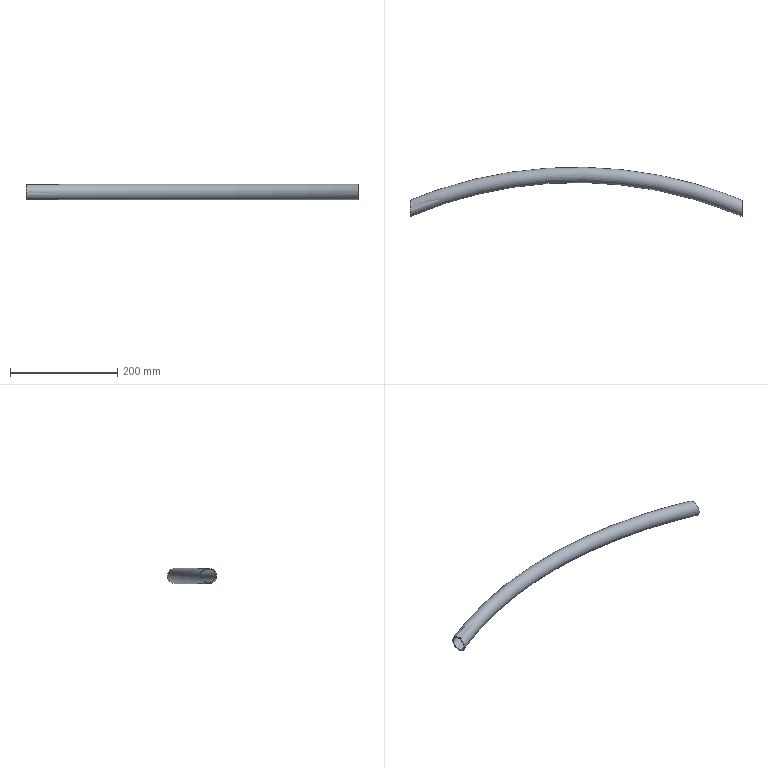Part | STEP file | 5091501 | 1 solid | 4 faces | box 620 x 92.341 x 28.6 mm | volume 81368 mm3 | torus 2 | plane 2